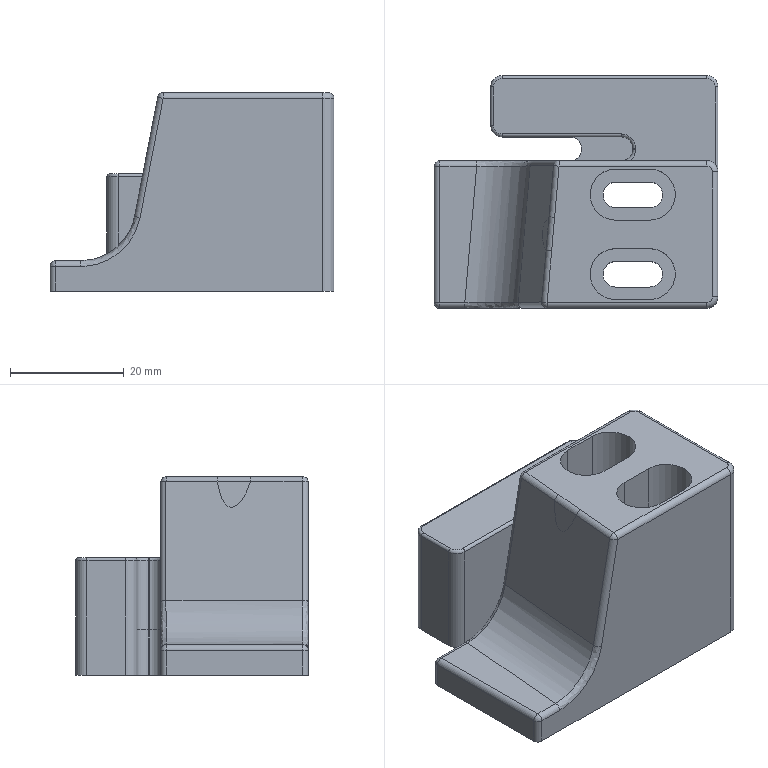NC program | NX | posted with a generic post | part box 50 x 41 x 35 mm
Lines 1 to 1812 of 6591:
N10 G17 G21 G94 G90
(CAVITY_MILL , TOOL : D10)
N12 T09 M6
N14 G54
N16 G17 G0 G90 X-34.997 Y3.062 S9500 M3
N18 G43 Z30. H9
N20 Z0.553
N22 G94 G1 Z-0.947 F1000.
N24 X-28.997 Y6.526
N26 G3 X-28.497 Y7.392 R1.
N28 G1 Y23.502 F3000.
N30 G2 X-28.003 Y23.997 R0.495
N32 G1 X28.003
N34 G2 X28.497 Y23.502 R0.495
N36 G1 Y9.717
N38 G2 X31.299 Y3.5 R8.299
N40 G1 Y-18.5
N42 G2 X23. Y-26.799 R8.299
N44 G1 X-5.157 Y-26.796
N46 X-5.288
N48 G2 X-6.39 Y-26.68 R7.299
N50 X-10.838 Y-23.997 R7.303
N52 G1 X-28.003
N54 G2 X-28.497 Y-23.502 R0.495
N56 G1 Y7.392
N58 X-22.497
N60 Y17.997
N62 X22.497
N64 Y11.799
N66 X-3.012 Y11.798
N68 X-3.265 Y11.793
N70 G3 X-4.303 Y11.679 R7.299
N72 X-10.27 Y5.134 R7.306
N74 G1 X-12.288 Y-17.997
N76 X-11.092 Y-18.101
N78 X-9.074 Y5.028
N80 G2 X-4.087 Y10.499 R6.106
N82 X-3.24 Y10.593 R6.099
N84 G1 X-2.987 Y10.599
N86 X23.
N88 G2 X30.099 Y3.5 R7.099
N90 G1 Y-18.5
N92 G2 X23. Y-25.599 R7.099
N94 G1 X-5.111 Y-25.596
N96 X-5.254
N98 G2 X-6.176 Y-25.5 R6.099
N100 X-11.168 Y-18.972 R6.103
N102 G1 X-11.092 Y-18.101
N104 X-12.288 Y-17.997
N106 X-22.497
N108 Y7.392
N110 X-16.497
N112 Y11.997
N114 X-13.98
N116 G3 X-16.247 Y5.658 R13.306
N118 G1 X-16.497 Y2.788
N120 X-16.715 Y-2.207
N122 G2 X-17.497 Y-2.111 R5.
N124 G1 Y-12.997
N126 X-16.87
N128 X-15.927 Y-2.179
N130 G2 X-16.715 Y-2.207 R5.
N132 G1 X-16.497 Y2.788
N134 Y7.392
N136 G3 X-16.997 Y8.258 R1.
N138 G1 Z0.553
N140 G0 X-34.997 Y4.111 Z-0.393
N142 G1 Z-1.893 F1000.
N144 X-28.997 Y7.575
N146 G3 X-28.497 Y8.441 R1.
N148 G1 Y23.502 F3000.
N150 G2 X-28.002 Y23.997 R0.495
N152 G1 X28.002
N154 G2 X28.497 Y23.502 R0.495
N156 G1 Y9.719
N158 G2 X31.3 Y3.5 R8.3
N160 G1 Y-18.5
N162 G2 X23. Y-26.8 R8.3
N164 G1 X-5.254
N166 G2 X-11.011 Y-23.997 R7.322
N168 G1 X-28.002
N170 G2 X-28.497 Y-23.502 R0.495
N172 G1 Y8.441
N174 X-22.497
N176 Y17.997
N178 X22.497
N180 Y11.8
N182 X-3.16
N184 G3 X-10.453 Y5.135 R7.312
N186 G1 X-12.471 Y-17.997
N188 X-11.275 Y-18.101
N190 X-9.257 Y5.028
N192 G2 X-3.16 Y10.6 R6.112
N194 G1 X23.
N196 G2 X30.1 Y3.5 R7.1
N198 G1 Y-18.5
N200 G2 X23. Y-25.6 R7.1
N202 G1 X-5.254
N204 G2 X-11.351 Y-18.972 R6.122
N206 G1 X-11.275 Y-18.101
N208 X-12.471 Y-17.997
N210 X-22.497
N212 Y8.441
N214 X-16.497
N216 Y11.997
N218 X-14.162
N220 G3 X-16.43 Y5.661 R13.312
N222 G1 X-16.497 Y4.885
N224 X-16.715 Y-0.11
N226 G2 X-17.497 Y-0.014 R5.
N228 G1 Y-12.997
N230 X-17.053
N232 X-15.927 Y-0.082
N234 G2 X-16.715 Y-0.11 R5.
N236 G1 X-16.497 Y4.885
N238 Y8.441
N240 G3 X-16.997 Y9.307 R1.
N242 G1 Z-0.393
N244 G0 X-34.997 Y4.963 Z-1.34
N246 G1 Z-2.84 F1000.
N248 X-28.997 Y8.427
N250 G3 X-28.497 Y9.293 R1.
N252 G1 Y23.502 F3000.
N254 G2 X-28.002 Y23.997 R0.495
N256 G1 X28.002
N258 G2 X28.497 Y23.502 R0.495
N260 G1 Y9.719
N262 G2 X31.3 Y3.5 R8.3
N264 G1 Y-18.5
N266 G2 X23. Y-26.8 R8.3
N268 G1 X-5.438
N270 G2 X-11.193 Y-23.997 R7.324
N272 G1 X-28.002
N274 G2 X-28.497 Y-23.502 R0.495
N276 G1 Y9.293
N278 X-22.497
N280 Y17.997
N282 X22.497
N284 Y11.8
N286 X-3.343
N288 G3 X-10.636 Y5.135 R7.312
N290 G1 X-12.654 Y-17.997
N292 X-11.458 Y-18.101
N294 X-9.44 Y5.028
N296 G2 X-3.343 Y10.6 R6.112
N298 G1 X23.
N300 G2 X30.1 Y3.5 R7.1
N302 G1 Y-18.5
N304 G2 X23. Y-25.6 R7.1
N306 G1 X-5.437
N308 G2 X-11.534 Y-18.972 R6.124
N310 G1 X-11.458 Y-18.101
N312 X-12.654 Y-17.997
N314 X-22.497
N316 Y9.293
N318 X-16.497
N320 Y11.997
N322 X-14.344
N324 G3 X-16.497 Y6.59 R13.312
N326 G1 X-17.497 Y1.691
N328 Y-12.997
N330 X-17.236
N332 X-15.961 Y1.619
N334 G2 X-17.497 Y1.691 R5.
N336 G1 X-16.497 Y6.59
N338 Y9.293
N340 G3 X-16.997 Y10.159 R1.
N342 G1 Z-1.34
N344 G0 X-34.997 Y5.428 Z-2.287
N346 G1 Z-3.787 F1000.
N348 X-28.997 Y8.892
N350 G3 X-28.497 Y9.758 R1.
N352 G1 Y23.502 F3000.
N354 G2 X-28.002 Y23.997 R0.495
N356 G1 X28.002
N358 G2 X28.497 Y23.502 R0.495
N360 G1 Y9.718
N362 G2 X31.3 Y3.5 R8.3
N364 G1 Y-18.5
N366 G2 X23. Y-26.8 R8.3
N368 G1 X-5.621
N370 G2 X-11.376 Y-23.997 R7.323
N372 G1 X-28.002
N374 G2 X-28.497 Y-23.502 R0.495
N376 G1 Y9.758
N378 X-22.497
N380 Y17.997
N382 X22.497
N384 Y11.8
N386 X-3.526
N388 G3 X-10.819 Y5.135 R7.312
N390 G1 X-12.837 Y-17.997
N392 X-11.641 Y-18.101
N394 X-9.623 Y5.028
N396 G2 X-3.526 Y10.6 R6.112
N398 G1 X23.
N400 G2 X30.1 Y3.5 R7.1
N402 G1 Y-18.5
N404 G2 X23. Y-25.6 R7.1
N406 G1 X-5.62
N408 G2 X-11.717 Y-18.972 R6.123
N410 G1 X-11.641 Y-18.101
N412 X-12.837 Y-17.997
N414 X-22.497
N416 Y9.758
N418 X-16.497
N420 Y11.997
N422 X-14.527
N424 G3 X-16.497 Y7.52 R13.312
N426 G1 X-17.497 Y2.621
N428 Y-12.997
N430 X-17.419
N432 X-16.064 Y2.539
N434 G2 X-17.497 Y2.621 R5.
N436 G1 X-16.497 Y7.52
N438 Y9.758
N440 G3 X-16.997 Y10.624 R1.
N442 G1 Z-2.287
N444 G0 X-19.934 Y30.497 Z-3.233
N446 G1 Z-4.733 F1000.
N448 X-16.47 Y24.497
N450 G3 X-15.604 Y23.997 R1.
N452 G1 X28.002 F3000.
N454 G2 X28.497 Y23.502 R0.495
N456 G1 Y9.718
N458 G2 X31.3 Y3.5 R8.3
N460 G1 Y-18.5
N462 G2 X23. Y-26.8 R8.3
N464 G1 X-5.803
N466 G2 X-11.56 Y-23.997 R7.322
N468 G1 X-28.002
N470 G2 X-28.497 Y-23.502 R0.495
N472 G1 Y23.502
N474 G2 X-28.002 Y23.997 R0.495
N476 G1 X-15.604
N478 Y17.997
N480 X22.497
N482 Y11.8
N484 X-3.709
N486 G3 X-11.002 Y5.135 R7.312
N488 G1 X-13.02 Y-17.997
N490 X-11.824 Y-18.101
N492 X-9.806 Y5.028
N494 G2 X-3.709 Y10.6 R6.112
N496 G1 X23.
N498 G2 X30.1 Y3.5 R7.1
N500 G1 Y-18.5
N502 G2 X23. Y-25.6 R7.1
N504 G1 X-5.803
N506 G2 X-11.9 Y-18.972 R6.122
N508 G1 X-11.824 Y-18.101
N510 X-13.02 Y-17.997
N512 X-22.497
N514 Y17.997
N516 X-15.604
N518 Y11.997
N520 X-14.71
N522 G3 X-16.497 Y8.217 R13.312
N524 G1 X-17.497 Y3.318
N526 Y-11.794
N528 X-16.187 Y3.226
N530 G2 X-17.497 Y3.318 R5.
N532 G1 X-16.497 Y8.217
N534 Y11.997
N536 X-15.604
N538 G3 X-14.738 Y12.497 R1.
N540 G1 Z-3.233
N542 G0 X-20.021 Y30.497 Z-4.18
N544 G1 Z-5.68 F1000.
N546 X-16.557 Y24.497
N548 G3 X-15.691 Y23.997 R1.
N550 G1 X28.002 F3000.
N552 G2 X28.498 Y23.502 R0.495
N554 G1 Y9.718
N556 G2 X31.3 Y3.5 R8.3
N558 G1 Y-18.5
N560 G2 X23. Y-26.8 R8.3
N562 G1 X-5.994
N564 G2 X-11.744 Y-23.997 R7.402
N566 G1 X-28.002
N568 G2 X-28.498 Y-23.502 R0.495
N570 G1 Y23.502
N572 G2 X-28.002 Y23.997 R0.495
N574 G1 X-15.691
N576 Y17.997
N578 X22.498
N580 Y11.8
N582 X-3.892
N584 G3 X-11.185 Y5.133 R7.333
N586 G1 X-13.203 Y-17.997
N588 X-12.007 Y-18.101
N590 X-9.989 Y5.028
N592 G2 X-3.892 Y10.6 R6.133
N594 G1 X23.
N596 G2 X30.1 Y3.5 R7.1
N598 G1 Y-18.5
N600 G2 X23. Y-25.6 R7.1
N602 G1 X-5.986
N604 G2 X-11.251 Y-22.607 R6.202
N606 X-12.087 Y-19.012 R5.948
N608 G1 X-12.007 Y-18.101
N610 X-13.203 Y-17.997
N612 X-22.498
N614 Y17.997
N616 X-15.691
N618 Y11.997
N620 X-14.885
N622 G3 X-16.498 Y8.782 R13.333
N624 G1 X-17.498 Y3.883
N626 Y-9.698
N628 X-16.321 Y3.785
N630 G2 X-17.498 Y3.883 R5.
N632 G1 X-16.498 Y8.782
N634 Y11.997
N636 X-15.691
N638 G3 X-14.825 Y12.497 R1.
N640 G1 Z-4.18
N642 G0 X-20.114 Y30.497 Z-5.127
N644 G1 Z-6.627 F1000.
N646 X-16.65 Y24.497
N648 G3 X-15.784 Y23.997 R1.
N650 G1 X28.002 F3000.
N652 G2 X28.498 Y23.502 R0.495
N654 G1 Y9.718
N656 G2 X31.3 Y3.5 R8.3
N658 G1 Y-18.5
N660 G2 X23. Y-26.8 R8.3
N662 G1 X-6.175
N664 G2 X-11.92 Y-23.997 R7.369
N666 G1 X-28.002
N668 G2 X-28.498 Y-23.502 R0.495
N670 G1 Y23.502
N672 G2 X-28.002 Y23.997 R0.495
N674 G1 X-15.784
N676 Y17.997
N678 X22.498
N680 Y11.8
N682 X-4.075
N684 G3 X-11.368 Y5.133 R7.329
N686 G1 X-13.386 Y-17.997
N688 X-12.19 Y-18.101
N690 X-10.172 Y5.028
N692 G2 X-4.075 Y10.6 R6.129
N694 G1 X23.
N696 G2 X30.1 Y3.5 R7.1
N698 G1 Y-18.5
N700 G2 X23. Y-25.6 R7.1
N702 G1 X-6.169
N704 G2 X-12.081 Y-21.076 R6.169
N706 X-12.27 Y-19.017 R5.826
N708 G1 X-12.19 Y-18.101
N710 X-13.386 Y-17.997
N712 X-22.498
N714 Y17.997
N716 X-15.784
N718 Y11.997
N720 X-15.07
N722 G3 X-16.498 Y9.286 R13.329
N724 G1 X-17.498 Y4.387
N726 Y-7.601
N728 X-16.461 Y4.286
N730 G2 X-17.498 Y4.387 R5.
N732 G1 X-16.498 Y9.286
N734 Y11.997
N736 X-15.784
N738 G3 X-14.918 Y12.497 R1.
N740 G1 Z-5.127
N742 G0 X-20.209 Y30.497 Z-6.073
N744 G1 Z-7.573 F1000.
N746 X-16.744 Y24.497
N748 G3 X-15.878 Y23.997 R1.
N750 G1 X28.002 F3000.
N752 G2 X28.498 Y23.502 R0.496
N754 G1 Y9.718
N756 G2 X31.3 Y3.5 R8.3
N758 G1 Y-18.5
N760 G2 X23. Y-26.8 R8.3
N762 G1 X-6.352
N764 G2 X-12.109 Y-23.997 R7.323
N766 G1 X-28.002
N768 G2 X-28.498 Y-23.502 R0.496
N770 G1 Y23.502
N772 G2 X-28.002 Y23.997 R0.496
N774 G1 X-15.878
N776 Y17.997
N778 X22.498
N780 Y11.8
N782 X-4.258
N784 G3 X-11.551 Y5.135 R7.312
N786 G1 X-13.569 Y-17.997
N788 X-12.373 Y-18.101
N790 X-10.355 Y5.028
N792 G2 X-4.258 Y10.6 R6.112
N794 G1 X23.
N796 G2 X30.1 Y3.5 R7.1
N798 G1 Y-18.5
N800 G2 X23. Y-25.6 R7.1
N802 G1 X-6.352
N804 G2 X-12.449 Y-18.972 R6.123
N806 G1 X-12.373 Y-18.101
N808 X-13.569 Y-17.997
N810 X-22.498
N812 Y17.997
N814 X-15.878
N816 Y11.997
N818 X-15.259
N820 G3 X-16.498 Y9.744 R13.312
N822 G1 X-17.498 Y4.845
N824 Y-5.504
N826 X-16.604 Y4.745
N828 G2 X-17.498 Y4.845 R5.
N830 G1 X-16.498 Y9.744
N832 Y11.997
N834 X-15.878
N836 G3 X-15.012 Y12.497 R1.
N838 G1 Z-6.073
N840 G0 X-20.297 Y30.497 Z-7.02
N842 G1 Z-8.52 F1000.
N844 X-16.833 Y24.497
N846 G3 X-15.967 Y23.997 R1.
N848 G1 X28.002 F3000.
N850 G2 X28.498 Y23.502 R0.496
N852 G1 Y9.718
N854 G2 X31.3 Y3.5 R8.3
N856 G1 Y-18.5
N858 G2 X23. Y-26.8 R8.3
N860 G1 X-6.534
N862 G2 X-12.3 Y-23.997 R7.309
N864 G1 X-28.002
N866 G2 X-28.498 Y-23.502 R0.496
N868 G1 Y23.502
N870 G2 X-28.002 Y23.997 R0.496
N872 G1 X-15.967
N874 Y17.997
N876 X22.498
N878 Y11.8
N880 X-4.441
N882 G3 X-11.734 Y5.133 R7.328
N884 G1 X-13.752 Y-17.997
N886 X-12.556 Y-18.102
N888 X-10.538 Y5.028
N890 G2 X-4.441 Y10.6 R6.128
N892 G1 X23.
N894 G2 X30.1 Y3.5 R7.1
N896 G1 Y-18.5
N898 G2 X23. Y-25.6 R7.1
N900 G1 X-6.535
N902 G2 X-12.632 Y-18.972 R6.109
N904 G1 X-12.556 Y-18.102
N906 X-13.752 Y-17.997
N908 X-22.498
N910 Y17.997
N912 X-15.967
N914 Y11.997
N916 X-15.436
N918 G3 X-16.498 Y10.141 R13.328
N920 G1 X-17.498 Y5.242
N922 Y-3.408
N924 X-16.751 Y5.148
N926 G2 X-17.498 Y5.242 R5.
N928 G1 X-16.498 Y10.141
N930 Y11.997
N932 X-15.967
N934 G3 X-15.101 Y12.497 R1.
N936 G1 Z-7.02
N938 G0 X-20.392 Y30.497 Z-7.967
N940 G1 Z-9.467 F1000.
N942 X-16.927 Y24.497
N944 G3 X-16.061 Y23.997 R1.
N946 G1 X28.002 F3000.
N948 G2 X28.498 Y23.502 R0.496
N950 G1 Y9.718
N952 G2 X31.3 Y3.5 R8.3
N954 G1 Y-18.5
N956 G2 X23. Y-26.8 R8.3
N958 G1 X-6.717
N960 G2 X-12.483 Y-23.997 R7.309
N962 G1 X-28.002
N964 G2 X-28.498 Y-23.502 R0.496
N966 G1 Y23.502
N968 G2 X-28.002 Y23.997 R0.496
N970 G1 X-16.061
N972 Y17.997
N974 X22.498
N976 Y11.8
N978 X-4.624
N980 G3 X-11.917 Y5.135 R7.312
N982 G1 X-13.935 Y-17.997
N984 X-12.739 Y-18.102
N986 X-10.721 Y5.028
N988 G2 X-4.624 Y10.6 R6.112
N990 G1 X23.
N992 G2 X30.1 Y3.5 R7.1
N994 G1 Y-18.5
N996 G2 X23. Y-25.6 R7.1
N998 G1 X-6.718
N1000 G2 X-12.815 Y-18.972 R6.109
N1002 G1 X-12.739 Y-18.102
N1004 X-13.935 Y-17.997
N1006 X-22.498
N1008 Y17.997
N1010 X-16.061
N1012 Y11.997
N1014 X-15.625
N1016 G3 X-16.498 Y10.525 R13.312
N1018 G1 X-17.299 Y3.281
N1020 X-16.498 Y10.525
N1022 Y11.997
N1024 X-16.061
N1026 G3 X-15.195 Y12.497 R1.
N1028 G1 Z-7.967
N1030 G0 X-20.483 Y30.497 Z-8.913
N1032 G1 Z-10.413 F1000.
N1034 X-17.019 Y24.497
N1036 G3 X-16.153 Y23.997 R1.
N1038 G1 X28.002 F3000.
N1040 G2 X28.498 Y23.502 R0.496
N1042 G1 Y9.718
N1044 G2 X31.3 Y3.5 R8.3
N1046 G1 Y-18.5
N1048 G2 X23. Y-26.8 R8.3
N1050 G1 X-6.902
N1052 G2 X-12.657 Y-23.997 R7.323
N1054 G1 X-28.002
N1056 G2 X-28.498 Y-23.502 R0.496
N1058 G1 Y23.502
N1060 G2 X-28.002 Y23.997 R0.496
N1062 G1 X-16.153
N1064 Y17.997
N1066 X22.498
N1068 Y11.8
N1070 X-4.807
N1072 G3 X-12.1 Y5.135 R7.312
N1074 G1 X-14.118 Y-17.997
N1076 X-12.922 Y-18.102
N1078 X-10.904 Y5.028
N1080 G2 X-4.807 Y10.6 R6.112
N1082 G1 X23.
N1084 G2 X30.1 Y3.5 R7.1
N1086 G1 Y-18.5
N1088 G2 X23. Y-25.6 R7.1
N1090 G1 X-6.901
N1092 G2 X-12.998 Y-18.972 R6.123
N1094 G1 X-12.922 Y-18.102
N1096 X-14.118 Y-17.997
N1098 X-22.498
N1100 Y17.997
N1102 X-16.153
N1104 Y11.997
N1106 X-15.808
N1108 G3 X-16.498 Y10.871 R13.312
N1110 G1 X-17.349 Y4.219
N1112 X-16.498 Y10.871
N1114 Y11.997
N1116 X-16.153
N1118 G3 X-15.287 Y12.497 R1.
N1120 G1 Z-8.913
N1122 G0 X-20.575 Y30.498 Z-9.86
N1124 G1 Z-11.36 F1000.
N1126 X-17.11 Y24.498
N1128 G3 X-16.244 Y23.998 R1.
N1130 G1 X28.002 F3000.
N1132 G2 X28.498 Y23.502 R0.496
N1134 G1 Y9.718
N1136 G2 X31.3 Y3.5 R8.3
N1138 G1 Y-18.5
N1140 G2 X23. Y-26.8 R8.3
N1142 G1 X-7.083
N1144 G2 X-12.849 Y-23.998 R7.309
N1146 G1 X-28.002
N1148 G2 X-28.498 Y-23.502 R0.496
N1150 G1 Y23.502
N1152 G2 X-28.002 Y23.998 R0.496
N1154 G1 X-16.244
N1156 Y17.998
N1158 X22.498
N1160 Y11.8
N1162 X-4.99
N1164 G3 X-12.283 Y5.135 R7.312
N1166 G1 X-14.301 Y-17.998
N1168 X-13.105 Y-18.102
N1170 X-11.087 Y5.028
N1172 G2 X-4.99 Y10.6 R6.112
N1174 G1 X23.
N1176 G2 X30.1 Y3.5 R7.1
N1178 G1 Y-18.5
N1180 G2 X23. Y-25.6 R7.1
N1182 G1 X-7.084
N1184 G2 X-13.181 Y-18.972 R6.109
N1186 G1 X-13.105 Y-18.102
N1188 X-14.301 Y-17.998
N1190 X-22.498
N1192 Y17.998
N1194 X-16.244
N1196 Y11.998
N1198 X-15.991
N1200 G3 X-16.498 Y11.195 R13.312
N1202 G1 X-17.399 Y5.149
N1204 X-16.498 Y11.195
N1206 Y11.998
N1208 X-16.244
N1210 G3 X-15.378 Y12.498 R1.
N1212 G1 Z-9.86
N1214 G0 X-20.666 Y30.498 Z-10.807
N1216 G1 Z-12.307 F1000.
N1218 X-17.202 Y24.498
N1220 G3 X-16.336 Y23.998 R1.
N1222 G1 X28.002 F3000.
N1224 G2 X28.498 Y23.501 R0.496
N1226 G1 Y9.718
N1228 G2 X31.3 Y3.5 R8.3
N1230 G1 Y-18.5
N1232 G2 X23. Y-26.8 R8.3
N1234 G1 X-7.266
N1236 G2 X-13.032 Y-23.998 R7.309
N1238 G1 X-28.002
N1240 G2 X-28.498 Y-23.501 R0.496
N1242 G1 Y23.501
N1244 G2 X-28.002 Y23.998 R0.496
N1246 G1 X-16.336
N1248 Y17.998
N1250 X22.498
N1252 Y11.8
N1254 X-5.173
N1256 G3 X-12.466 Y5.135 R7.312
N1258 G1 X-14.484 Y-17.998
N1260 X-13.288 Y-18.102
N1262 X-11.27 Y5.028
N1264 G2 X-5.173 Y10.6 R6.112
N1266 G1 X23.
N1268 G2 X30.1 Y3.5 R7.1
N1270 G1 Y-18.5
N1272 G2 X23. Y-25.6 R7.1
N1274 G1 X-7.267
N1276 G2 X-13.364 Y-18.972 R6.109
N1278 G1 X-13.288 Y-18.102
N1280 X-14.484 Y-17.998
N1282 X-22.498
N1284 Y17.998
N1286 X-16.336
N1288 Y11.998
N1290 X-16.174
N1292 G3 X-16.498 Y11.499 R13.312
N1294 G1 X-17.442 Y6.081
N1296 X-16.498 Y11.499
N1298 Y11.998
N1300 X-16.336
N1302 G3 X-15.47 Y12.498 R1.
N1304 G1 Z-10.807
N1306 G0 X-20.758 Y30.498 Z-11.753
N1308 G1 Z-13.253 F1000.
N1310 X-17.293 Y24.498
N1312 G3 X-16.427 Y23.998 R1.
N1314 G1 X28.002 F3000.
N1316 G2 X28.498 Y23.501 R0.496
N1318 G1 Y9.718
N1320 G2 X31.3 Y3.5 R8.3
N1322 G1 Y-18.5
N1324 G2 X23. Y-26.8 R8.3
N1326 G1 X-7.45
N1328 G2 X-13.206 Y-23.998 R7.322
N1330 G1 X-28.002
N1332 G2 X-28.498 Y-23.501 R0.496
N1334 G1 Y23.501
N1336 G2 X-28.002 Y23.998 R0.496
N1338 G1 X-16.427
N1340 Y17.998
N1342 X22.498
N1344 Y11.8
N1346 X-5.356
N1348 G3 X-12.649 Y5.135 R7.312
N1350 G1 X-14.667 Y-17.998
N1352 X-13.471 Y-18.102
N1354 X-11.453 Y5.028
N1356 G2 X-5.356 Y10.6 R6.112
N1358 G1 X23.
N1360 G2 X30.1 Y3.5 R7.1
N1362 G1 Y-18.5
N1364 G2 X23. Y-25.6 R7.1
N1366 G1 X-7.45
N1368 G2 X-13.547 Y-18.972 R6.122
N1370 G1 X-13.471 Y-18.102
N1372 X-14.667 Y-17.998
N1374 X-22.498
N1376 Y17.998
N1378 X-16.427
N1380 Y11.998
N1382 X-16.357
N1384 G3 X-16.498 Y11.786 R13.312
N1386 G1 X-17.48 Y6.782
N1388 X-16.498 Y11.786
N1390 Y11.998
N1392 X-16.427
N1394 G3 X-15.561 Y12.498 R1.
N1396 G1 Z-11.753
N1398 G0 X-34.998 Y1.255 Z-12.7
N1400 G1 Z-14.2 F1000.
N1402 X-28.998 Y4.719
N1404 G3 X-28.498 Y5.585 R1.
N1406 G1 Y23.501 F3000.
N1408 G2 X-28.002 Y23.998 R0.496
N1410 G1 X28.002
N1412 G2 X28.498 Y23.501 R0.496
N1414 G1 Y9.718
N1416 G2 X31.3 Y3.5 R8.3
N1418 G1 Y-18.5
N1420 G2 X23. Y-26.8 R8.3
N1422 G1 X-7.632
N1424 G2 X-13.389 Y-23.998 R7.321
N1426 G1 X-28.002
N1428 G2 X-28.498 Y-23.501 R0.496
N1430 G1 Y5.585
N1432 X-22.498
N1434 Y17.998
N1436 X22.498
N1438 Y11.8
N1440 X-5.391
N1442 G3 X-12.83 Y5.133 R7.322
N1444 G1 X-14.848 Y-17.998
N1446 X-13.653 Y-18.102
N1448 X-11.635 Y5.028
N1450 G2 X-5.403 Y10.6 R6.122
N1452 G1 X23.
N1454 G2 X30.1 Y3.5 R7.1
N1456 G1 Y-18.5
N1458 G2 X23. Y-25.6 R7.1
N1460 G1 X-7.631
N1462 G2 X-13.728 Y-18.972 R6.121
N1464 G1 X-13.653 Y-18.102
N1466 X-14.848 Y-17.998
N1468 X-22.498
N1470 Y5.585
N1472 X-17.998
N1474 Y13.498
N1476 X-13.181
N1478 G3 X-17.313 Y5.529 R11.822
N1480 G1 X-17.998 Y-2.329
N1482 Y5.585
N1484 G3 X-18.498 Y6.451 R1.
N1486 G1 Z-12.7
N1488 G0 X-34.998 Y-4.476 Z-13.65
N1490 G1 Z-15.15 F1000.
N1492 X-28.998 Y-1.012
N1494 G3 X-28.498 Y-0.146 R1.
N1496 G1 Y23.501 F3000.
N1498 G2 X-28.002 Y23.998 R0.497
N1500 G1 X-19.218
N1502 G2 X-13. Y26.8 R8.3
N1504 G1 X23.
N1506 G2 X31.3 Y18.5 R8.3
N1508 G1 Y-18.5
N1510 G2 X23. Y-26.8 R8.3
N1512 G1 X-7.817
N1514 G2 X-13.573 Y-23.998 R7.323
N1516 G1 X-28.002
N1518 G2 X-28.498 Y-23.501 R0.497
N1520 G1 Y-0.146
N1522 X-22.498
N1524 Y17.998
N1526 X-21.3
N1528 Y11.7
N1530 G3 X-13.166 Y3.402 R8.3
N1532 G1 X-15.033 Y-17.998
N1534 X-13.838 Y-18.102
N1536 X-11.857 Y4.6
N1538 X-13.
N1540 G2 X-20.1 Y11.7 R7.1
N1542 G1 Y18.5
N1544 G2 X-13. Y25.6 R7.1
N1546 G1 X23.
N1548 G2 X30.1 Y18.5 R7.1
N1550 G1 Y-18.5
N1552 G2 X23. Y-25.6 R7.1
N1554 G1 X-7.816
N1556 G2 X-13.914 Y-18.972 R6.123
N1558 G1 X-13.838 Y-18.102
N1560 X-15.033 Y-17.998
N1562 X-22.498
N1564 Y-0.146
N1566 X-17.998
N1568 Y-0.084
N1570 X-17.988 Y-0.088
N1572 X-17.998 Y-0.208
N1574 Y-0.146
N1576 G3 X-18.498 Y0.72 R1.
N1578 G1 Z-13.65
N1580 G0 X-34.998 Y-4.33 Z-14.6
N1582 G1 Z-16.1 F1000.
N1584 X-28.998 Y-0.866
N1586 G3 X-28.498 Y0. R1.
N1588 G1 Y23.501 F3000.
N1590 G2 X-28.002 Y23.998 R0.497
N1592 G1 X-19.218
N1594 G2 X-13. Y26.8 R8.3
N1596 G1 X23.
N1598 G2 X31.3 Y18.5 R8.3
N1600 G1 Y-18.5
N1602 G2 X23. Y-26.8 R8.3
N1604 G1 X-8.
N1606 G2 X-13.758 Y-23.998 R7.32
N1608 G1 X-28.002
N1610 G2 X-28.498 Y-23.501 R0.497
N1612 G1 Y0.
N1614 X-22.498
N1616 Y17.998
N1618 X-21.3
N1620 Y11.7
N1622 G3 X-13.349 Y3.407 R8.3
N1624 G1 X-15.217 Y-17.998
N1626 X-14.021 Y-18.102
N1628 X-12.041 Y4.6
N1630 X-13.
N1632 G2 X-20.1 Y11.7 R7.1
N1634 G1 Y18.5
N1636 G2 X-13. Y25.6 R7.1
N1638 G1 X23.
N1640 G2 X30.1 Y18.5 R7.1
N1642 G1 Y-18.5
N1644 G2 X23. Y-25.6 R7.1
N1646 G1 X-8.
N1648 G2 X-14.097 Y-18.972 R6.12
N1650 G1 X-14.021 Y-18.102
N1652 X-15.217 Y-17.998
N1654 X-22.498
N1656 Y0.
N1658 G3 X-22.998 Y0.866 R1.
N1660 G1 X-34.998
N1662 Z-14.6
N1664 G0 Y-4.33 Z-15.55
N1666 G1 Z-17.05 F1000.
N1668 X-28.998 Y-0.866
N1670 G3 X-28.498 Y0. R1.
N1672 G1 Y23.501 F3000.
N1674 G2 X-28.002 Y23.998 R0.497
N1676 G1 X-19.218
N1678 G2 X-13. Y26.8 R8.3
N1680 G1 X23.
N1682 G2 X31.3 Y18.5 R8.3
N1684 G1 Y-18.5
N1686 G2 X23. Y-26.8 R8.3
N1688 G1 X-8.184
N1690 G2 X-13.941 Y-23.998 R7.321
N1692 G1 X-28.002
N1694 G2 X-28.498 Y-23.501 R0.497
N1696 G1 Y0.
N1698 X-22.498
N1700 Y17.998
N1702 X-21.3
N1704 Y11.7
N1706 G3 X-13.532 Y3.417 R8.3
N1708 G1 X-15.4 Y-17.998
N1710 X-14.205 Y-18.102
N1712 X-12.225 Y4.6
N1714 X-13.
N1716 G2 X-20.1 Y11.7 R7.1
N1718 G1 Y18.5
N1720 G2 X-13. Y25.6 R7.1
N1722 G1 X23.
N1724 G2 X30.1 Y18.5 R7.1
N1726 G1 Y-18.5
N1728 G2 X23. Y-25.6 R7.1
N1730 G1 X-8.184
N1732 G2 X-14.281 Y-18.972 R6.121
N1734 G1 X-14.205 Y-18.102
N1736 X-15.4 Y-17.998
N1738 X-22.498
N1740 Y0.
N1742 G3 X-22.998 Y0.866 R1.
N1744 G1 X-34.998
N1746 Z-15.55
N1748 G0 X-34.999 Y-4.33 Z-16.5
N1750 G1 Z-18. F1000.
N1752 X-28.999 Y-0.866
N1754 G3 X-28.499 Y0. R1.
N1756 G1 Y23.501 F3000.
N1758 G2 X-28.002 Y23.998 R0.497
N1760 G1 X-19.218
N1762 G2 X-13. Y26.8 R8.3
N1764 G1 X23.
N1766 G2 X31.3 Y18.5 R8.3
N1768 G1 Y-18.5
N1770 G2 X23. Y-26.8 R8.3
N1772 G1 X-8.332
N1774 G2 X-14.123 Y-23.998 R7.324
N1776 G1 X-28.002
N1778 G2 X-28.499 Y-23.501 R0.497
N1780 G1 Y0.
N1782 X-22.499
N1784 Y17.998
N1786 X-21.3
N1788 Y11.7
N1790 G3 X-13.715 Y3.431 R8.3
N1792 G1 X-15.584 Y-17.998
N1794 X-14.389 Y-18.103
N1796 X-12.408 Y4.6
N1798 X-13.
N1800 G2 X-20.1 Y11.7 R7.1
N1802 G1 Y18.5
N1804 G2 X-13. Y25.6 R7.1
N1806 G1 X23.
N1808 G2 X30.1 Y18.5 R7.1
N1810 G1 Y-18.5
N1812 G2 X23. Y-25.6 R7.1
N1814 G1 X-8.334
N1816 G2 X-14.464 Y-18.972 R6.124
N1818 G1 X-14.389 Y-18.103
N1820 X-15.584 Y-17.998
N1822 X-22.499
N1824 Y0.
N1826 G3 X-22.999 Y0.866 R1.
N1828 G1 X-34.999
N1830 Z-16.5
N1832 G0 Y-4.33 Z-17.45
N1834 G1 Z-18.95 F1000.
N1836 X-28.999 Y-0.866
N1838 G3 X-28.499 Y0. R1.
N1840 G1 Y23.501 F3000.
N1842 G2 X-28.001 Y23.998 R0.497
N1844 G1 X-19.218
N1846 G2 X-13. Y26.8 R8.3
N1848 G1 X23.
N1850 G2 X31.3 Y18.5 R8.3
N1852 G1 Y-18.5
N1854 G2 X23. Y-26.8 R8.3
N1856 G1 X-8.552
N1858 G2 X-14.307 Y-23.998 R7.322
N1860 G1 X-28.001
N1862 G2 X-28.499 Y-23.501 R0.497
N1864 G1 Y0.
N1866 X-22.499
N1868 Y17.998
N1870 X-21.3
N1872 Y11.7
N1874 G3 X-13.897 Y3.449 R8.3
N1876 G1 X-15.768 Y-17.998
N1878 X-14.572 Y-18.103
N1880 X-12.592 Y4.6
N1882 X-13.
N1884 G2 X-20.1 Y11.7 R7.1
N1886 G1 Y18.5
N1888 G2 X-13. Y25.6 R7.1
N1890 G1 X23.
N1892 G2 X30.1 Y18.5 R7.1
N1894 G1 Y-18.5
N1896 G2 X23. Y-25.6 R7.1
N1898 G1 X-8.551
N1900 G2 X-14.648 Y-18.972 R6.122
N1902 G1 X-14.572 Y-18.103
N1904 X-15.768 Y-17.998
N1906 X-22.499
N1908 Y0.
N1910 G3 X-22.999 Y0.866 R1.
N1912 G1 X-34.999
N1914 Z-17.45
N1916 G0 Y-4.33 Z-18.4
N1918 G1 Z-19.9 F1000.
N1920 X-28.999 Y-0.866
N1922 G3 X-28.499 Y0. R1.
N1924 G1 Y23.501 F3000.
N1926 G2 X-28.001 Y23.998 R0.497
N1928 G1 X-19.217
N1930 G2 X-13. Y26.8 R8.3
N1932 G1 X23.
N1934 G2 X31.3 Y18.5 R8.3
N1936 G1 Y-18.5
N1938 G2 X23. Y-26.8 R8.3
N1940 G1 X-8.733
N1942 G2 X-14.493 Y-23.998 R7.317
N1944 G1 X-28.001
N1946 G2 X-28.499 Y-23.501 R0.497
N1948 G1 Y0.
N1950 X-22.499
N1952 Y17.998
N1954 X-21.3
N1956 Y11.7
N1958 G3 X-14.077 Y3.47 R8.3
N1960 G1 X-15.95 Y-17.998
N1962 X-14.755 Y-18.103
N1964 X-12.774 Y4.6
N1966 X-13.
N1968 G2 X-20.1 Y11.7 R7.1
N1970 G1 Y18.5
N1972 G2 X-13. Y25.6 R7.1
N1974 G1 X23.
N1976 G2 X30.1 Y18.5 R7.1
N1978 G1 Y-18.5
N1980 G2 X23. Y-25.6 R7.1
N1982 G1 X-8.733
N1984 G2 X-14.83 Y-18.972 R6.117
N1986 G1 X-14.755 Y-18.103
N1988 X-15.95 Y-17.998
N1990 X-22.499
N1992 Y0.
N1994 G3 X-22.999 Y0.866 R1.
N1996 G1 X-34.999
N1998 Z-18.4
N2000 G0 Y-4.33 Z-19.4
N2002 G1 Z-20.9 F1000.
N2004 X-28.999 Y-0.866
N2006 G3 X-28.499 Y0. R1.
N2008 G1 Y23.501 F3000.
N2010 G2 X-28.001 Y23.999 R0.497
N2012 G1 X-19.217
N2014 G2 X-13. Y26.8 R8.3
N2016 G1 X23.
N2018 G2 X31.3 Y18.5 R8.3
N2020 G1 Y-18.5
N2022 G2 X23. Y-26.8 R8.3
N2024 G1 X-8.927
N2026 G2 X-14.692 Y-23.999 R7.309
N2028 G1 X-28.001
N2030 G2 X-28.499 Y-23.501 R0.497
N2032 G1 Y0.
N2034 X-22.499
N2036 Y17.999
N2038 X-21.3
N2040 Y11.7
N2042 G3 X-14.269 Y3.498 R8.3
N2044 G1 X-16.145 Y-17.999
N2046 X-14.949 Y-18.103
N2048 X-12.969 Y4.6
N2050 X-13.
N2052 G2 X-20.1 Y11.7 R7.1
N2054 G1 Y18.5
N2056 G2 X-13. Y25.6 R7.1
N2058 G1 X23.
N2060 G2 X30.1 Y18.5 R7.1
N2062 G1 Y-18.5
N2064 G2 X23. Y-25.6 R7.1
N2066 G1 X-8.928
N2068 G2 X-15.025 Y-18.972 R6.109
N2070 G1 X-14.949 Y-18.103
N2072 X-16.145 Y-17.999
N2074 X-22.499
N2076 Y0.
N2078 G3 X-22.999 Y0.866 R1.
N2080 G1 X-34.999
N2082 Z-19.4
N2084 G0 Y-4.33 Z-20.4
N2086 G1 Z-21.9 F1000.
N2088 X-28.999 Y-0.866
N2090 G3 X-28.499 Y0. R1.
N2092 G1 Y23.501 F3000.
N2094 G2 X-28.001 Y23.999 R0.498
N2096 G1 X-19.217
N2098 G2 X-13. Y26.8 R8.3
N2100 G1 X23.
N2102 G2 X31.3 Y18.5 R8.3
N2104 G1 Y-18.5
N2106 G2 X23. Y-26.8 R8.3
N2108 G1 X-9.12
N2110 G2 X-14.886 Y-23.999 R7.309
N2112 G1 X-28.001
N2114 G2 X-28.499 Y-23.501 R0.498
N2116 G1 Y0.
N2118 X-22.499
N2120 Y17.999
N2122 X-21.3
N2124 Y11.7
N2126 G3 X-14.461 Y3.53 R8.3
N2128 G1 X-16.339 Y-17.999
N2130 X-15.143 Y-18.103
N2132 X-13.162 Y4.602
N2134 G2 X-20.1 Y11.7 R7.1
N2136 G1 Y18.5
N2138 G2 X-13. Y25.6 R7.1
N2140 G1 X23.
N2142 G2 X30.1 Y18.5 R7.1
N2144 G1 Y-18.5
N2146 G2 X23. Y-25.6 R7.1
N2148 G1 X-9.121
N2150 G2 X-15.219 Y-18.972 R6.109
N2152 G1 X-15.143 Y-18.103
N2154 X-16.339 Y-17.999
N2156 X-22.499
N2158 Y0.
N2160 G3 X-22.999 Y0.866 R1.
N2162 G1 X-34.999
N2164 Z-20.4
N2166 G0 Y-4.33 Z-21.4
N2168 G1 Z-22.9 F1000.
N2170 X-28.999 Y-0.866
N2172 G3 X-28.499 Y0. R1.
N2174 G1 Y23.501 F3000.
N2176 G2 X-28.001 Y23.999 R0.498
N2178 G1 X-19.217
N2180 G2 X-13. Y26.8 R8.3
N2182 G1 X23.
N2184 G2 X31.3 Y18.5 R8.3
N2186 G1 Y-18.5
N2188 G2 X23. Y-26.8 R8.3
N2190 G1 X-9.354
N2192 G2 X-15.142 Y-23.999 R7.319
N2194 G1 X-28.001
N2196 G2 X-28.499 Y-23.501 R0.498
N2198 G1 Y0.
N2200 X-22.499
N2202 Y17.999
N2204 X-21.3
N2206 Y11.7
N2208 G3 X-14.719 Y3.58 R8.3
N2210 G1 X-16.601 Y-17.999
N2212 X-15.406 Y-18.103
N2214 X-13.424 Y4.613
N2216 G2 X-20.1 Y11.7 R7.1
N2218 G1 Y18.5
N2220 G2 X-13. Y25.6 R7.1
N2222 G1 X23.
N2224 G2 X30.1 Y18.5 R7.1
N2226 G1 Y-18.5
N2228 G2 X23. Y-25.6 R7.1
N2230 G1 X-9.357
N2232 G2 X-15.482 Y-18.975 R6.119
N2234 G1 X-15.406 Y-18.103
N2236 X-16.601 Y-17.999
N2238 X-22.499
N2240 Y0.
N2242 G3 X-22.999 Y0.866 R1.
N2244 G1 X-34.999
N2246 Z-21.4
N2248 G0 Y-4.33 Z-22.4
N2250 G1 Z-23.9 F1000.
N2252 X-28.999 Y-0.866
N2254 G3 X-28.499 Y0. R1.
N2256 G1 Y23.501 F3000.
N2258 G2 X-28.001 Y23.999 R0.498
N2260 G1 X-19.217
N2262 G2 X-13. Y26.8 R8.3
N2264 G1 X23.
N2266 G2 X31.3 Y18.5 R8.3
N2268 G1 Y-18.5
N2270 G2 X23. Y-26.8 R8.3
N2272 G1 X-9.696
N2274 G2 X-15.52 Y-23.999 R7.429
N2276 G1 X-28.001
N2278 G2 X-28.499 Y-23.501 R0.498
N2280 G1 Y0.
N2282 X-22.499
N2284 Y17.999
N2286 X-21.3
N2288 Y11.7
N2290 G3 X-15.096 Y3.669 R8.3
N2292 G1 X-16.987 Y-17.999
N2294 X-15.791 Y-18.103
N2296 X-13.807 Y4.646
N2298 G2 X-20.1 Y11.7 R7.1
N2300 G1 Y18.5
N2302 G2 X-13. Y25.6 R7.1
N2304 G1 X23.
N2306 G2 X30.1 Y18.5 R7.1
N2308 G1 Y-18.5
N2310 G2 X23. Y-25.6 R7.1
N2312 G1 X-9.697
N2314 G2 X-15.031 Y-22.607 R6.229
N2316 X-15.868 Y-18.979 R5.934
N2318 G1 X-15.791 Y-18.103
N2320 X-16.987 Y-17.999
N2322 X-22.499
N2324 Y0.
N2326 G3 X-22.999 Y0.866 R1.
N2328 G1 X-34.999
N2330 Z-22.4
N2332 G0 Y-4.33 Z-23.4
N2334 G1 Z-24.9 F1000.
N2336 X-28.999 Y-0.866
N2338 G3 X-28.499 Y0. R1.
N2340 G1 Y23.501 F3000.
N2342 G2 X-28.001 Y23.999 R0.498
N2344 G1 X-19.217
N2346 G2 X-13. Y26.8 R8.3
N2348 G1 X23.
N2350 G2 X31.3 Y18.5 R8.3
N2352 G1 Y-18.5
N2354 G2 X23. Y-26.8 R8.3
N2356 G1 X-10.159
N2358 G2 X-15.896 Y-24.157 R7.602
N2360 X-16.029 Y-23.999 R7.047
N2362 G1 X-28.001
N2364 G2 X-28.499 Y-23.501 R0.498
N2366 G1 Y0.
N2368 X-22.499
N2370 Y17.999
N2372 X-21.3
N2374 Y11.7
N2376 G3 X-15.609 Y3.821 R8.3
N2378 G1 X-17.512 Y-17.999
N2380 X-16.317 Y-18.103
N2382 X-14.325 Y4.725
N2384 G2 X-20.1 Y11.7 R7.1
N2386 G1 Y18.5
N2388 G2 X-13. Y25.6 R7.1
N2390 G1 X23.
N2392 G2 X30.1 Y18.5 R7.1
N2394 G1 Y-18.5
N2396 G2 X23. Y-25.6 R7.1
N2398 G1 X-10.156
N2400 G2 X-14.988 Y-23.373 R6.402
N2402 X-16.394 Y-18.984 R5.847
N2404 G1 X-16.317 Y-18.103
N2406 X-17.512 Y-17.999
N2408 X-22.499
N2410 Y0.
N2412 G3 X-22.999 Y0.866 R1.
N2414 G1 X-34.999
N2416 Z-23.4
N2418 G0 Y-4.33 Z-24.4
N2420 G1 Z-25.9 F1000.
N2422 X-28.999 Y-0.866
N2424 G3 X-28.499 Y0. R1.
N2426 G1 Y23.501 F3000.
N2428 G2 X-28.001 Y23.999 R0.498
N2430 G1 X-19.217
N2432 G2 X-13. Y26.8 R8.3
N2434 G1 X23.
N2436 G2 X31.3 Y18.5 R8.3
N2438 G1 Y-18.5
N2440 G2 X23. Y-26.8 R8.3
N2442 G1 X-10.778
N2444 G2 X-14.254 Y-25.974 R8.44
N2446 X-16.71 Y-23.999 R7.638
N2448 G1 X-28.001
N2450 G2 X-28.499 Y-23.501 R0.498
N2452 G1 Y0.
N2454 X-22.499
N2456 Y17.999
N2458 X-21.3
N2460 Y11.7
N2462 G3 X-16.282 Y4.077 R8.3
N2464 G1 X-18.208 Y-17.999
N2466 X-17.013 Y-18.103
N2468 X-15.007 Y4.889
N2470 G2 X-20.1 Y11.7 R7.1
N2472 G1 Y18.5
N2474 G2 X-13. Y25.6 R7.1
N2476 G1 X23.
N2478 G2 X30.1 Y18.5 R7.1
N2480 G1 Y-18.5
N2482 G2 X23. Y-25.6 R7.1
N2484 G1 X-10.754
N2486 G2 X-13.711 Y-24.904 R7.24
N2488 X-16.653 Y-21.842 R6.438
N2490 X-17.09 Y-18.991 R5.953
N2492 G1 X-17.013 Y-18.103
N2494 X-18.208 Y-17.999
N2496 X-22.499
N2498 Y0.
N2500 G3 X-22.999 Y0.866 R1.
N2502 G1 X-34.999
N2504 Z-24.4
N2506 G0 Y-4.33 Z-25.4
N2508 G1 Z-26.9 F1000.
N2510 X-28.999 Y-0.866
N2512 G3 X-28.499 Y0. R1.
N2514 G1 Y23.501 F3000.
N2516 G2 X-28.001 Y23.999 R0.498
N2518 G1 X-19.217
N2520 G2 X-13. Y26.8 R8.3
N2522 G1 X23.
N2524 G2 X31.3 Y18.5 R8.3
N2526 G1 Y-18.5
N2528 G2 X23. Y-26.8 R8.3
N2530 G1 X-11.51
N2532 G2 X-17.462 Y-24.17 R8.083
N2534 X-17.61 Y-23.999 R6.978
N2536 G1 X-28.001
N2538 G2 X-28.499 Y-23.501 R0.498
N2540 G1 Y0.
N2542 X-22.499
N2544 Y17.999
N2546 X-21.3
N2548 Y11.7
N2550 G3 X-17.155 Y4.515 R8.3
N2552 G1 X-19.119 Y-17.999
N2554 X-17.924 Y-18.103
N2556 X-15.913 Y4.95
N2558 X-15.887 Y5.213
N2560 G2 X-20.1 Y11.7 R7.1
N2562 G1 Y18.5
N2564 G2 X-13. Y25.6 R7.1
N2566 G1 X23.
N2568 G2 X30.1 Y18.5 R7.1
N2570 G1 Y-18.5
N2572 G2 X23. Y-25.6 R7.1
N2574 G1 X-11.508
N2576 G2 X-16.566 Y-23.373 R6.883
N2578 X-18.002 Y-19. R5.778
N2580 G1 X-17.924 Y-18.103
N2582 X-19.119 Y-17.999
N2584 X-22.499
N2586 Y0.
N2588 G3 X-22.999 Y0.866 R1.
N2590 G1 X-34.999
N2592 Z-25.4
N2594 G0 Y-4.33 Z-26.267
N2596 G1 Z-27.767 F1000.
N2598 X-28.999 Y-0.866
N2600 G3 X-28.499 Y0. R1.
N2602 G1 Y23.501 F3000.
N2604 G2 X-28.001 Y23.999 R0.498
N2606 G1 X-19.217
N2608 G2 X-13. Y26.8 R8.3
N2610 G1 X23.
N2612 G2 X31.3 Y18.5 R8.3
N2614 G1 Y-18.5
N2616 G2 X23. Y-26.8 R8.3
N2618 G1 X-12.35
N2620 G2 X-18.473 Y-24.193 R8.441
N2622 X-18.647 Y-23.999 R6.777
N2624 G1 X-28.001
N2626 G2 X-28.499 Y-23.501 R0.498
N2628 G1 Y0.
N2630 X-22.499
N2632 Y17.999
N2634 X-21.3
N2636 Y11.7
N2638 G3 X-18.163 Y5.201 R8.3
N2640 G1 X-18.176 Y5.094
N2642 X-20.191 Y-17.999
N2644 X-18.995 Y-18.104
N2646 X-16.981 Y4.989
N2648 X-16.877 Y5.752
N2650 G2 X-20.1 Y11.7 R7.1
N2652 G1 Y18.5
N2654 G2 X-13. Y25.6 R7.1
N2656 G1 X23.
N2658 G2 X30.1 Y18.5 R7.1
N2660 G1 Y-18.5
N2662 G2 X23. Y-25.6 R7.1
N2664 G1 X-12.352
N2666 G2 X-17.597 Y-23.373 R7.241
N2668 X-19.074 Y-19.011 R5.577
N2670 G1 X-18.995 Y-18.104
N2672 X-20.191 Y-17.999
N2674 X-22.499
N2676 Y0.
N2678 G3 X-22.999 Y0.866 R1.
N2680 G1 X-34.999
N2682 Z-26.267
N2684 G0 Y-4.33 Z-27.133
N2686 G1 Z-28.633 F1000.
N2688 X-28.999 Y-0.866
N2690 G3 X-28.499 Y0. R1.
N2692 G1 Y23.501 F3000.
N2694 G2 X-28.001 Y23.999 R0.499
N2696 G1 X-19.217
N2698 G2 X-13. Y26.8 R8.3
N2700 G1 X23.
N2702 G2 X31.3 Y18.5 R8.3
N2704 G1 Y-18.5
N2706 G2 X23. Y-26.8 R8.3
N2708 G1 X-13.414
N2710 G2 X-19.269 Y-24.772 R9.284
N2712 X-20.103 Y-23.999 R6.589
N2714 G1 X-28.001
N2716 G2 X-28.499 Y-23.501 R0.499
N2718 G1 Y0.
N2720 X-22.499
N2722 Y17.999
N2724 X-21.3
N2726 Y11.7
N2728 G3 X-19.423 Y6.443 R8.3
N2730 G1 X-19.67 Y5.211
N2732 X-19.689 Y5.079
N2734 X-21.703 Y-17.999
N2736 X-20.507 Y-18.104
N2738 X-18.494 Y4.974
N2740 X-18.191 Y6.481
N2742 X-18.087 Y6.747
N2744 G2 X-20.1 Y11.7 R7.1
N2746 G1 Y18.5
N2748 G2 X-13. Y25.6 R7.1
N2750 G1 X23.
N2752 G2 X30.1 Y18.5 R7.1
N2754 G1 Y-18.5
N2756 G2 X23. Y-25.6 R7.1
N2758 G1 X-13.419
N2760 G2 X-18.526 Y-23.829 R8.084
N2762 X-20.588 Y-19.026 R5.389
N2764 G1 X-20.507 Y-18.104
N2766 X-21.703 Y-17.999
N2768 X-22.499
N2770 Y0.
N2772 G3 X-22.999 Y0.866 R1.
N2774 G1 X-34.999
N2776 Z-27.133
N2778 G0 X-35. Y8.34 Z-28.
N2780 G1 Z-29.5 F1000.
N2782 X-29. Y11.805
N2784 G3 X-28.5 Y12.671 R1.
N2786 G1 Y23.501 F3000.
N2788 G2 X-28.001 Y23.999 R0.499
N2790 G1 X-19.217
N2792 G2 X-13. Y26.8 R8.3
N2794 G1 X23.
N2796 G2 X31.3 Y18.5 R8.3
N2798 G1 Y-18.5
N2800 G2 X23. Y-26.8 R8.3
N2802 G1 X-14.9 Y-26.799
N2804 G2 X-21.439 Y-25.313 R17.601
N2806 X-23.386 Y-23.999 R6.619
N2808 G1 X-28.001
N2810 G2 X-28.5 Y-23.501 R0.499
N2812 G1 Y12.671
N2814 X-22.5
N2816 Y17.999
N2818 X-21.3
N2820 Y11.7
N2822 G3 X-20.934 Y9.263 R8.3
N2824 X-22.5 Y7.342 R7.048
N2826 G1 X-21.45 Y6.759
N2828 G2 X-19.499 Y8.84 R5.848
N2830 X-20.1 Y11.7 R7.1
N2832 G1 Y18.5
N2834 G2 X-13. Y25.6 R7.1
N2836 G1 X23.
N2838 G2 X30.1 Y18.5 R7.1
N2840 G1 Y-18.5
N2842 G2 X23. Y-25.6 R7.1
N2844 G1 X-14.861
N2846 G2 X-20.955 Y-24.215 R16.401
N2848 X-24.167 Y-18.786 R5.419
N2850 G1 X-22.099 Y4.924
N2852 G2 X-21.45 Y6.759 R5.848
N2854 G1 X-22.5 Y7.342
N2856 Y12.671
N2858 G3 X-23. Y13.537 R1.
N2860 G1 X-35.
N2862 Z-28.
N2864 G0 Y10.562 Z-28.917
N2866 G1 Z-30.417 F1000.
N2868 X-29. Y14.026
N2870 G3 X-28.5 Y14.892 R1.
N2872 G1 Y23.501 F3000.
N2874 G2 X-28.001 Y24. R0.499
N2876 G1 X-19.217
N2878 G2 X-13. Y26.8 R8.3
N2880 G1 X23.
N2882 G2 X31.3 Y18.5 R8.3
N2884 G1 Y-18.5
N2886 G2 X23. Y-26.8 R8.3
N2888 G1 X-17.644
N2890 X-19.28 Y-26.771
N2892 X-19.589 Y-26.785
N2894 X-24.
N2896 G2 X-31.285 Y-19.5 R7.285
N2898 G1 Y4.5
N2900 G2 X-28.5 Y10.229 R7.285
N2902 G1 Y14.892
N2904 X-22.5
N2906 Y18.
N2908 X-21.3
N2910 Y11.785
N2912 X-22.5
N2914 Y10.585
N2916 X-20.012
N2918 G2 X-20.1 Y11.7 R7.1
N2920 G1 Y18.5
N2922 G2 X-13. Y25.6 R7.1
N2924 G1 X23.
N2926 G2 X30.1 Y18.5 R7.1
N2928 G1 Y-18.5
N2930 G2 X23. Y-25.6 R7.1
N2932 G1 X-17.623
N2934 X-19.298 Y-25.571
N2936 X-19.589 Y-25.585
N2938 X-24.
N2940 G2 X-30.085 Y-19.5 R6.085
N2942 G1 Y4.5
N2944 G2 X-24. Y10.585 R6.085
N2946 G1 X-22.5
N2948 Y11.785
N2950 Y14.892
N2952 G3 X-23. Y15.758 R1.
N2954 G1 X-35.
N2956 Z-28.917
N2958 G0 Y10.57 Z-29.833
N2960 G1 Z-31.333 F1000.
N2962 X-29. Y14.034
N2964 G3 X-28.5 Y14.9 R1.
N2966 G1 Y23.501 F3000.
N2968 G2 X-28.001 Y24. R0.499
N2970 G1 X-19.216
N2972 G2 X-13. Y26.8 R8.3
N2974 G1 X23.
N2976 G2 X31.3 Y18.5 R8.3
N2978 G1 Y-18.5
N2980 G2 X23. Y-26.8 R8.3
N2982 G1 X-24.
N2984 G2 X-31.3 Y-19.5 R7.3
N2986 G1 Y4.5
N2988 G2 X-28.5 Y10.248 R7.3
N2990 G1 Y14.9
N2992 X-22.5
N2994 Y18.
N2996 X-21.3
N2998 Y11.8
N3000 X-22.5
N3002 Y10.6
N3004 X-20.014
N3006 G2 X-20.1 Y11.7 R7.1
N3008 G1 Y18.5
N3010 G2 X-13. Y25.6 R7.1
N3012 G1 X23.
N3014 G2 X30.1 Y18.5 R7.1
N3016 G1 Y-18.5
N3018 G2 X23. Y-25.6 R7.1
N3020 G1 X-24.
N3022 G2 X-30.1 Y-19.5 R6.1
N3024 G1 Y4.5
N3026 G2 X-24. Y10.6 R6.1
N3028 G1 X-22.5
N3030 Y11.8
N3032 Y14.9
N3034 G3 X-23. Y15.766 R1.
N3036 G1 X-35.
N3038 Z-29.833
N3040 G0 Y10.57 Z-30.75
N3042 G1 Z-32.25 F1000.
N3044 X-29. Y14.034
N3046 G3 X-28.5 Y14.9 R1.
N3048 G1 Y23.501 F3000.
N3050 G2 X-28.001 Y24. R0.499
N3052 G1 X-19.216
N3054 G2 X-13. Y26.8 R8.3
N3056 G1 X23.
N3058 G2 X31.3 Y18.5 R8.3
N3060 G1 Y-18.5
N3062 G2 X23. Y-26.8 R8.3
N3064 G1 X-24.
N3066 G2 X-31.3 Y-19.5 R7.3
N3068 G1 Y4.5
N3070 G2 X-28.5 Y10.248 R7.3
N3072 G1 Y14.9
N3074 X-22.5
N3076 Y18.
N3078 X-21.3
N3080 Y11.8
N3082 X-22.5
N3084 Y10.6
N3086 X-20.014
N3088 G2 X-20.1 Y11.7 R7.1
N3090 G1 Y18.5
N3092 G2 X-13. Y25.6 R7.1
N3094 G1 X23.
N3096 G2 X30.1 Y18.5 R7.1
N3098 G1 Y-18.5
N3100 G2 X23. Y-25.6 R7.1
N3102 G1 X-24.
N3104 G2 X-30.1 Y-19.5 R6.1
N3106 G1 Y4.5
N3108 G2 X-24. Y10.6 R6.1
N3110 G1 X-22.5
N3112 Y11.8
N3114 Y14.9
N3116 G3 X-23. Y15.766 R1.
N3118 G1 X-35.
N3120 Z-30.75
N3122 G0 Y10.57 Z-31.667
N3124 G1 Z-33.167 F1000.
N3126 X-29. Y14.034
N3128 G3 X-28.5 Y14.9 R1.
N3130 G1 Y23.501 F3000.
N3132 G2 X-28.001 Y24. R0.499
N3134 G1 X-19.216
N3136 G2 X-13. Y26.8 R8.3
N3138 G1 X23.
N3140 G2 X31.3 Y18.5 R8.3
N3142 G1 Y-18.5
N3144 G2 X23. Y-26.8 R8.3
N3146 G1 X-24.
N3148 G2 X-31.3 Y-19.5 R7.3
N3150 G1 Y4.5
N3152 G2 X-28.5 Y10.248 R7.3
N3154 G1 Y14.9
N3156 X-22.5
N3158 Y18.
N3160 X-21.3
N3162 Y11.8
N3164 X-22.5
N3166 Y10.6
N3168 X-20.014
N3170 G2 X-20.1 Y11.7 R7.1
N3172 G1 Y18.5
N3174 G2 X-13. Y25.6 R7.1
N3176 G1 X23.
N3178 G2 X30.1 Y18.5 R7.1
N3180 G1 Y-18.5
N3182 G2 X23. Y-25.6 R7.1
N3184 G1 X-24.
N3186 G2 X-30.1 Y-19.5 R6.1
N3188 G1 Y4.5
N3190 G2 X-24. Y10.6 R6.1
N3192 G1 X-22.5
N3194 Y11.8
N3196 Y14.9
N3198 G3 X-23. Y15.766 R1.
N3200 G1 X-35.
N3202 Z-31.667
N3204 G0 Y10.57 Z-32.583
N3206 G1 Z-34.083 F1000.
N3208 X-29. Y14.034
N3210 G3 X-28.5 Y14.9 R1.
N3212 G1 Y23.501 F3000.
N3214 G2 X-28.001 Y24. R0.499
N3216 G1 X-19.216
N3218 G2 X-13. Y26.8 R8.3
N3220 G1 X23.
N3222 G2 X31.3 Y18.5 R8.3
N3224 G1 Y-18.5
N3226 G2 X23. Y-26.8 R8.3
N3228 G1 X-24.
N3230 G2 X-31.3 Y-19.5 R7.3
N3232 G1 Y4.5
N3234 G2 X-28.5 Y10.248 R7.3
N3236 G1 Y14.9
N3238 X-22.5
N3240 Y18.
N3242 X-21.3
N3244 Y11.8
N3246 X-22.5
N3248 Y10.6
N3250 X-20.014
N3252 G2 X-20.1 Y11.7 R7.1
N3254 G1 Y18.5
N3256 G2 X-13. Y25.6 R7.1
N3258 G1 X23.
N3260 G2 X30.1 Y18.5 R7.1
N3262 G1 Y-18.5
N3264 G2 X23. Y-25.6 R7.1
N3266 G1 X-24.
N3268 G2 X-30.1 Y-19.5 R6.1
N3270 G1 Y4.5
N3272 G2 X-24. Y10.6 R6.1
N3274 G1 X-22.5
N3276 Y11.8
N3278 Y14.9
N3280 G3 X-23. Y15.766 R1.
N3282 G1 X-35.
N3284 Z-32.583
N3286 G0 Y10.57 Z-33.5
N3288 G1 Z-35. F1000.
N3290 X-29. Y14.034
N3292 G3 X-28.5 Y14.9 R1.
N3294 G1 Y23.501 F3000.
N3296 G2 X-28.001 Y24. R0.499
N3298 G1 X-19.216
N3300 G2 X-13. Y26.8 R8.3
N3302 G1 X23.
N3304 G2 X31.3 Y18.5 R8.3
N3306 G1 Y-18.5
N3308 G2 X23. Y-26.8 R8.3
N3310 G1 X-24.
N3312 G2 X-31.3 Y-19.5 R7.3
N3314 G1 Y4.5
N3316 G2 X-28.5 Y10.248 R7.3
N3318 G1 Y14.9
N3320 X-22.5
N3322 Y18.
N3324 X-21.3
N3326 Y11.8
N3328 X-22.5
N3330 Y10.6
N3332 X-20.014
N3334 G2 X-20.1 Y11.7 R7.1
N3336 G1 Y18.5
N3338 G2 X-13. Y25.6 R7.1
N3340 G1 X23.
N3342 G2 X30.1 Y18.5 R7.1
N3344 G1 Y-18.5
N3346 G2 X23. Y-25.6 R7.1
N3348 G1 X-24.
N3350 G2 X-30.1 Y-19.5 R6.1
N3352 G1 Y4.5
N3354 G2 X-24. Y10.6 R6.1
N3356 G1 X-22.5
N3358 Y11.8
N3360 Y14.9
N3362 G3 X-23. Y15.766 R1.
N3364 G1 X-35.
N3366 Z-33.5
N3368 G0 Z30.
N3370 M5
(ZLEVEL_PROFILE_COPY_COPY , TOOL : D10JING)
N3372 T10 M6
N3374 G54
N3376 G17 G0 G90 X24.645 Y-27.348 S9500 M3
N3378 G43 Z30. H10
N3380 Z-16.
N3382 G94 G1 Z-17.5 F1000.
N3384 X23.866 Y-26.
N3386 G3 X23. Y-25.5 R1.
N3388 G1 X-24. F1200.
N3390 G2 X-30. Y-19.5 R6.
N3392 G1 Y4.5
N3394 G2 X-24. Y10.5 R6.
N3396 G1 X-19.896
N3398 G2 X-20. Y11.7 R7.
N3400 G1 Y18.5
N3402 G2 X-13. Y25.5 R7.
N3404 G1 X23.
N3406 G2 X30. Y18.5 R7.
N3408 G1 Y-18.5
N3410 G2 X23. Y-25.5 R7.
N3412 G3 X22.134 Y-26. R1.
N3414 G1 X21.268 Y-27.5
N3416 Z-16.
N3418 G0 Z30.
N3420 X24.645 Y-27.348
N3422 Z-33.5
N3424 G1 Z-35. F1000.
N3426 X23.866 Y-26.
N3428 G3 X23. Y-25.5 R1.
N3430 G1 X-24. F1200.
N3432 G2 X-30. Y-19.5 R6.
N3434 G1 Y4.5
N3436 G2 X-24. Y10.5 R6.
N3438 G1 X-19.896
N3440 G2 X-20. Y11.7 R7.
N3442 G1 Y18.5
N3444 G2 X-13. Y25.5 R7.
N3446 G1 X23.
N3448 G2 X30. Y18.5 R7.
N3450 G1 Y-18.5
N3452 G2 X23. Y-25.5 R7.
N3454 G3 X22.134 Y-26. R1.
N3456 G1 X21.268 Y-27.5
N3458 Z-33.5
N3460 G0 Z30.
(FLOOR_WALL_1 , TOOL : D10JING)
N3462 X-20.556 Y21.128
N3464 Z-12.8
N3466 G1 Z-14.3 F1000.
N3468 X-20.191 Y20.497
N3470 G3 X-19.325 Y19.997 R1.
N3472 G1 X29.325
N3474 G2 X29.5 Y18.5 R6.5
N3476 G1 Y17.099
N3478 X-19.5
N3480 Y14.2
N3482 X29.5
N3484 Y11.302
N3486 X-19.488
N3488 G3 X-13. Y5.2 R6.5
N3490 G1 X-12.038
N3492 X-12.036 Y5.243
N3494 X-11.998 Y5.683
N3496 X-11.972 Y5.803
N3498 X-11.199 Y8.028
N3500 G2 X-11.067 Y8.231 R0.5
N3502 G1 X-8.889 Y10.245
N3504 G2 X-8.68 Y10.36 R0.5
N3506 G1 X-6.41 Y10.974
N3508 X-6.285 Y10.991
N3510 X-5.596 Y11.
N3512 X-5.589
N3514 X23.
N3516 G2 X28.675 Y8.403 R7.5
N3518 G1 X29.5
N3520 G3 X30.366 Y8.903 R1.
N3522 G1 X31. Y10.001
N3524 Z-12.8
N3526 G0 Z30.
N3528 X-13.533 Y3.718
N3530 Z-12.8
N3532 G1 Z-14.3
N3534 X-12.112 Y4.381
N3536 G3 X-11.538 Y5.2 R1.
N3538 G1 X-11.5 Y5.639
N3540 X-10.727 Y7.864
N3542 X-8.549 Y9.877
N3544 X-6.279 Y10.491
N3546 X-5.589 Y10.5
N3548 X23.
N3550 G2 X29.47 Y6.172 R7.
N3552 G3 X30.263 Y5.562 R1.
N3554 G1 X31.279 Y5.427
N3556 Z-12.8
N3558 G0 Z30.
N3560 X-28.553 Y-26.
N3562 Z-28.1
N3564 G1 Z-29.6
N3566 X-27.095 Y-25.319
N3568 G3 X-26.522 Y-24.5 R1.
N3570 G1 X-23.565 Y9.5
N3572 X-22.582
N3574 X-25.539 Y-24.5
N3576 G2 X-26.112 Y-25.319 R1.
N3578 G1 X-27.569 Y-26.
N3580 Z-28.1
N3582 G0 Z30.
N3584 X-19.493 Y-26.328
N3586 Z-28.1
N3588 G1 Z-29.6
N3590 X-19.751 Y-25.202
N3592 G3 X-20.432 Y-24.47 R1.
N3594 G1 X-24.914 Y-23.092
N3596 X-22.185 Y8.287
N3598 X-19.505 Y9.115
N3600 G2 X-19.645 Y9.5 R7.
N3602 G3 X-20.392 Y10.165 R1.
N3604 G1 X-24.43 Y11.
N3606 Z-28.1
N3608 G0 Z30.
N3610 M5